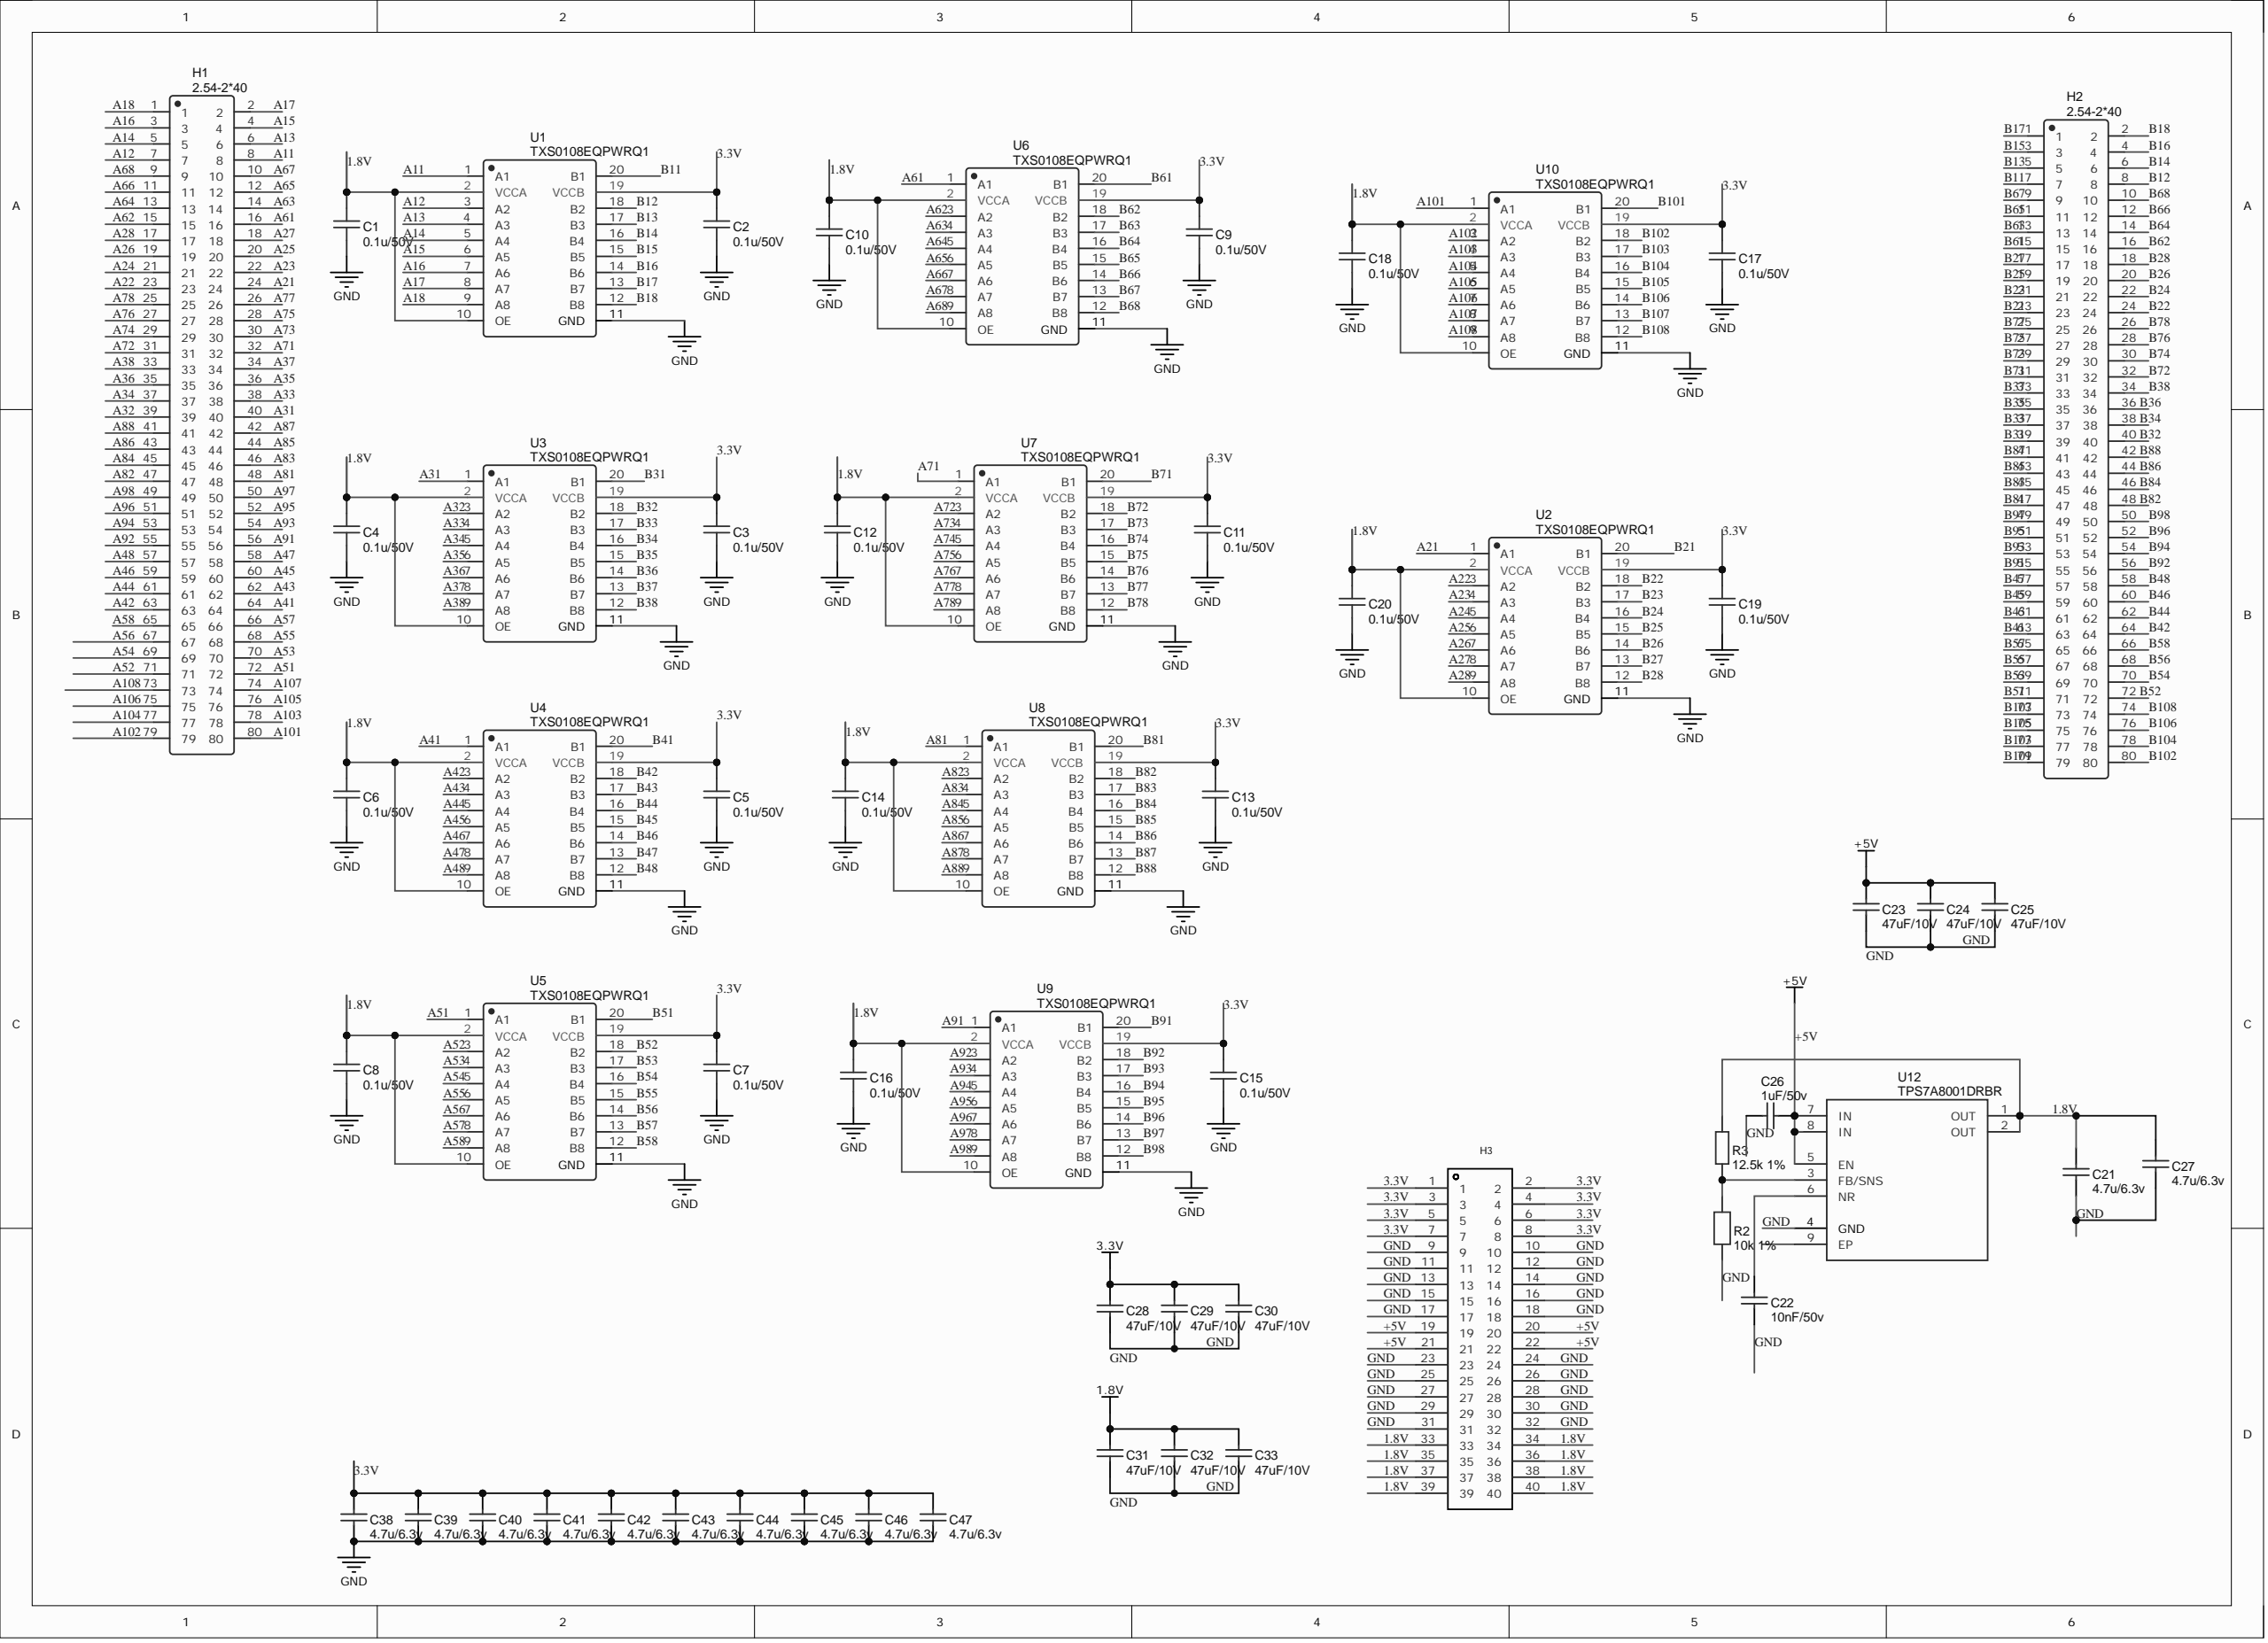Circuit board | Altium Designer | 59 parts | 166 nets
Bill of materials:
Comment,Description,Designator,Footprint,LibRef,Quantity
"0.1u/50V","","C1, C2, C3, C4, C5, C6, C7, C8, C9, C10, C11, C12, C13, C14, C15, C16, C17, C18, C19, C20","C0603","0.1u","20"
"4.7u/6.3v","","C21, C27, C38, C39, C40, C41, C42, C43, C44, C45, C46, C47","C0603","4.7u","12"
"10nF/50v","","C22","C0603","10nF","1"
"47uF/10V","","C23, C24, C25, C28, C29, C30, C31, C32, C33","C1206","4.7uF","9"
"1uF/50v","","C26","C0603","1uF","1"
"2.54-2*40","","H1, H2","HDR-TH_80P-P2.54-V-M-R2-C40-S2.54","2.54-2*40","2"
"B-2100S40P-B110","","H3","HDR-TH_40P-P2.54-V-M-R2-C20-S2.54","B-2100S40P-B110","1"
"10k 1%","","R2","R0603","","1"
"12.5k 1%","","R3","R0603","","1"
"TXS0108EQPWRQ1","","U1, U2, U3, U4, U5, U6, U7, U8, U9, U10","TSSOP-20_L6.5-W4.4-P0.65-LS6.4-BL","TXS0108EQPWRQ1","10"
"TPS7A8001DRBR","","U12","VSON-8_L3.0-W3.0-P0.65-TL-EP","TPS7A8001DRBR","1"
Netlist (Protel format):
[
C1
C0603
0.1u/50V



]
[
C2
C0603
0.1u/50V



]
[
C3
C0603
0.1u/50V



]
[
C4
C0603
0.1u/50V



]
[
C5
C0603
0.1u/50V



]
[
C6
C0603
0.1u/50V



]
[
C7
C0603
0.1u/50V



]
[
C8
C0603
0.1u/50V



]
[
C9
C0603
0.1u/50V



]
[
C10
C0603
0.1u/50V



]
[
C11
C0603
0.1u/50V



]
[
C12
C0603
0.1u/50V



]
[
C13
C0603
0.1u/50V



]
[
C14
C0603
0.1u/50V



]
[
C15
C0603
0.1u/50V



]
[
C16
C0603
0.1u/50V



]
[
C17
C0603
0.1u/50V



]
[
C18
C0603
0.1u/50V



]
[
C19
C0603
0.1u/50V



]
[
C20
C0603
0.1u/50V



]
[
C21
C0603
4.7u/6.3v



]
[
C22
C0603
10nF/50v



]
[
C23
C1206
47uF/10V



]
[
C24
C1206
47uF/10V



]
[
C25
C1206
47uF/10V



]
[
C26
C0603
1uF/50v



]
[
C27
C0603
4.7u/6.3v



]
[
C28
C1206
47uF/10V



]
[
C29
C1206
47uF/10V



]
[
C30
C1206
47uF/10V



]
[
C31
C1206
47uF/10V



]
[
C32
C1206
47uF/10V



]
[
C33
C1206
47uF/10V



]
[
C38
C0603
4.7u/6.3v



]
[
C39
C0603
4.7u/6.3v



]
[
C40
C0603
4.7u/6.3v



]
[
C41
C0603
4.7u/6.3v



]
[
C42
C0603
4.7u/6.3v



]
[
C43
C0603
4.7u/6.3v



]
[
C44
C0603
4.7u/6.3v



]
[
C45
C0603
4.7u/6.3v



]
[
C46
C0603
4.7u/6.3v



]
[
C47
C0603
4.7u/6.3v



]
[
H1
HDR-TH_80P-P2.54-V-M-R2-C40-S2.54
2.54-2*40



]
[
H2
HDR-TH_80P-P2.54-V-M-R2-C40-S2.54
2.54-2*40



]
[
H3
HDR-TH_40P-P2.54-V-M-R2-C20-S2.54
B-2100S40P-B110



]
[
R2
R0603
10k 1%



]
[
R3
R0603
12.5k 1%



]
[
U1
TSSOP-20_L6.5-W4.4-P0.65-LS6.4-BL
TXS0108EQPWRQ1



]
[
U2
TSSOP-20_L6.5-W4.4-P0.65-LS6.4-BL
TXS0108EQPWRQ1



]
[
U3
TSSOP-20_L6.5-W4.4-P0.65-LS6.4-BL
TXS0108EQPWRQ1



]
[
U4
TSSOP-20_L6.5-W4.4-P0.65-LS6.4-BL
TXS0108EQPWRQ1



]
[
U5
TSSOP-20_L6.5-W4.4-P0.65-LS6.4-BL
TXS0108EQPWRQ1



]
[
U6
TSSOP-20_L6.5-W4.4-P0.65-LS6.4-BL
TXS0108EQPWRQ1



]
[
U7
TSSOP-20_L6.5-W4.4-P0.65-LS6.4-BL
TXS0108EQPWRQ1



]
[
U8
TSSOP-20_L6.5-W4.4-P0.65-LS6.4-BL
TXS0108EQPWRQ1



]
[
U9
TSSOP-20_L6.5-W4.4-P0.65-LS6.4-BL
TXS0108EQPWRQ1



]
[
U10
TSSOP-20_L6.5-W4.4-P0.65-LS6.4-BL
TXS0108EQPWRQ1



]
[
U12
VSON-8_L3.0-W3.0-P0.65-TL-EP
TPS7A8001DRBR



]
(
NetR2_2
R2-2
R3-2
U12-3
)
(
NetC22_2
C22-2
U12-6
)
(
GND
C1-1
C2-1
C3-1
C4-1
C5-1
C6-1
C7-1
C8-1
C9-1
C10-1
C11-1
C12-1
C13-1
C14-1
C15-1
C16-1
C17-1
C18-1
C19-1
C20-1
C21-1
C22-1
C23-1
C24-1
C25-1
C26-2
C27-1
C28-1
C29-1
C30-1
C31-1
C32-1
C33-1
C38-1
C39-1
C40-1
C41-1
C42-1
C43-1
C44-1
C45-1
C46-1
C47-1
H3-9
H3-10
H3-11
H3-12
H3-13
H3-14
H3-15
H3-16
H3-17
H3-18
H3-23
H3-24
H3-25
H3-26
H3-27
H3-28
H3-29
H3-30
H3-31
H3-32
R2-1
U1-11
U2-11
U3-11
U4-11
U5-11
U6-11
U7-11
U8-11
U9-11
U10-11
U12-4
)
(
B108
H2-74
U10-12
)
(
B107
H2-73
U10-13
)
(
B106
H2-76
U10-14
)
(
B105
H2-75
U10-15
)
(
B104
H2-78
U10-16
)
(
B103
H2-77
U10-17
)
(
B102
H2-80
U10-18
)
(
B101
H2-79
U10-20
)
(
B98
H2-50
U9-12
)
(
B97
H2-49
U9-13
)
(
B96
H2-52
U9-14
)
(
B95
H2-51
U9-15
)
(
B94
H2-54
U9-16
)
(
B93
H2-53
U9-17
)
(
B92
H2-56
U9-18
)
(
B91
H2-55
U9-20
)
(
B88
H2-42
U8-12
)
(
B87
H2-41
U8-13
)
(
B86
H2-44
U8-14
)
(
B85
H2-43
U8-15
)
(
B84
H2-46
U8-16
)
(
B83
H2-45
U8-17
)
(
B82
H2-48
U8-18
)
(
B81
H2-47
U8-20
)
(
B78
H2-26
U7-12
)
(
B77
H2-25
U7-13
)
(
B76
H2-28
U7-14
)
(
B75
H2-27
U7-15
)
(
B74
H2-30
U7-16
)
(
B73
H2-29
U7-17
)
(
B72
H2-32
U7-18
)
(
B71
H2-31
U7-20
)
(
B68
H2-10
U6-12
)
(
B67
H2-9
U6-13
)
(
B66
H2-12
U6-14
)
(
B65
H2-11
U6-15
)
(
B64
H2-14
U6-16
)
(
B63
H2-13
U6-17
)
(
B62
H2-16
U6-18
)
(
B61
H2-15
U6-20
)
(
B58
H2-66
U5-12
)
(
B57
H2-65
U5-13
)
(
B56
H2-68
U5-14
)
(
B55
H2-67
U5-15
)
(
B54
H2-70
U5-16
)
(
B53
H2-69
U5-17
)
(
B52
H2-72
U5-18
)
(
B51
H2-71
U5-20
)
(
B48
H2-58
U4-12
)
(
B47
H2-57
U4-13
)
(
B46
H2-60
U4-14
)
(
B45
H2-59
U4-15
)
(
B44
H2-62
U4-16
)
(
B43
H2-61
U4-17
)
(
B42
H2-64
U4-18
)
(
B41
H2-63
U4-20
)
(
B38
H2-34
U3-12
)
(
B37
H2-33
U3-13
)
(
B36
H2-36
U3-14
)
(
B35
H2-35
U3-15
)
(
B34
H2-38
U3-16
)
(
B33
H2-37
U3-17
)
(
B32
H2-40
U3-18
)
(
B31
H2-39
U3-20
)
(
B28
H2-18
U2-12
)
(
B27
H2-17
U2-13
)
(
B26
H2-20
U2-14
)
(
B25
H2-19
U2-15
)
(
B24
H2-22
U2-16
)
(
B23
H2-21
U2-17
)
(
B22
H2-24
U2-18
)
(
B21
H2-23
U2-20
)
(
B18
H2-2
U1-12
)
(
B17
H2-1
U1-13
)
(
B16
H2-4
U1-14
)
(
B15
H2-3
U1-15
)
(
B14
H2-6
U1-16
)
(
B13
H2-5
U1-17
)
(
B12
H2-8
U1-18
)
(
B11
H2-7
U1-20
)
(
A108
H1-73
U10-9
)
(
A107
H1-74
U10-8
)
(
A106
H1-75
U10-7
)
(
A105
H1-76
U10-6
)
(
A104
H1-77
U10-5
)
(
A103
H1-78
U10-4
)
(
A102
H1-79
U10-3
)
(
A101
H1-80
U10-1
)
(
A98
H1-49
U9-9
)
(
A97
H1-50
U9-8
)
(
A96
H1-51
U9-7
)
(
A95
H1-52
U9-6
)
(
A94
H1-53
U9-5
)
(
A93
H1-54
U9-4
)
(
A92
H1-55
U9-3
)
(
A91
H1-56
U9-1
)
(
A88
H1-41
U8-9
)
(
A87
H1-42
U8-8
)
(
A86
H1-43
U8-7
)
(
A85
H1-44
U8-6
)
(
A84
H1-45
U8-5
)
(
A83
H1-46
U8-4
)
(
A82
H1-47
U8-3
)
(
A81
H1-48
U8-1
)
(
A78
H1-25
U7-9
)
(
A77
H1-26
U7-8
)
(
A76
H1-27
U7-7
)
(
A75
H1-28
U7-6
)
(
A74
H1-29
U7-5
)
(
A73
H1-30
U7-4
)
(
A72
H1-31
U7-3
)
(
A71
H1-32
U7-1
)
(
A68
H1-9
U6-9
)
(
A67
H1-10
U6-8
)
(
A66
H1-11
U6-7
)
(
A65
H1-12
U6-6
)
(
A64
H1-13
U6-5
)
(
A63
H1-14
U6-4
)
(
A62
H1-15
U6-3
)
(
A61
H1-16
U6-1
)
(
A58
H1-65
U5-9
)
(
A57
H1-66
U5-8
)
(
A56
H1-67
U5-7
)
(
A55
H1-68
U5-6
)
(
A54
H1-69
U5-5
)
(
A53
H1-70
U5-4
)
(
A52
H1-71
U5-3
)
(
A51
H1-72
U5-1
)
(
A48
H1-57
U4-9
)
(
A47
H1-58
U4-8
)
(
A46
H1-59
U4-7
)
(
A45
H1-60
U4-6
)
(
A44
H1-61
U4-5
)
(
A43
H1-62
U4-4
)
(
A42
H1-63
U4-3
)
(
A41
H1-64
U4-1
)
(
A38
H1-33
U3-9
)
(
A37
H1-34
U3-8
)
(
A36
H1-35
U3-7
)
(
A35
H1-36
U3-6
)
(
A34
H1-37
U3-5
)
(
A33
H1-38
U3-4
)
(
A32
H1-39
U3-3
)
(
A31
H1-40
U3-1
)
(
A28
H1-17
U2-9
)
(
A27
H1-18
U2-8
)
(
A26
H1-19
U2-7
)
(
A25
H1-20
U2-6
)
(
A24
H1-21
U2-5
)
(
A23
H1-22
U2-4
)
(
A22
H1-23
U2-3
)
(
A21
H1-24
U2-1
)
(
A18
H1-1
U1-9
)
(
A17
H1-2
U1-8
)
(
A16
H1-3
U1-7
)
(
A15
H1-4
U1-6
)
(
A14
H1-5
U1-5
)
(
A13
H1-6
U1-4
)
(
A12
H1-7
U1-3
)
(
A11
H1-8
U1-1
)
(
+5V
C23-2
C24-2
C25-2
C26-1
H3-19
H3-20
H3-21
H3-22
U12-5
U12-7
U12-8
)
(
3.3V
C2-2
C3-2
C5-2
C7-2
C9-2
C11-2
C13-2
C15-2
C17-2
C19-2
C28-2
C29-2
C30-2
C38-2
C39-2
C40-2
C41-2
C42-2
C43-2
C44-2
C45-2
C46-2
C47-2
H3-1
H3-2
H3-3
H3-4
H3-5
H3-6
H3-7
H3-8
U1-19
U2-19
U3-19
U4-19
U5-19
U6-19
U7-19
U8-19
U9-19
U10-19
)
(
1.8V
C1-2
C4-2
C6-2
C8-2
C10-2
C12-2
C14-2
C16-2
C18-2
C20-2
C21-2
C27-2
C31-2
C32-2
C33-2
H3-33
H3-34
H3-35
H3-36
H3-37
H3-38
H3-39
H3-40
R3-1
U1-2
U1-10
U2-2
U2-10
U3-2
U3-10
U4-2
U4-10
U5-2
U5-10
U6-2
U6-10
U7-2
U7-10
U8-2
U8-10
U9-2
U9-10
U10-2
U10-10
U12-1
U12-2
)